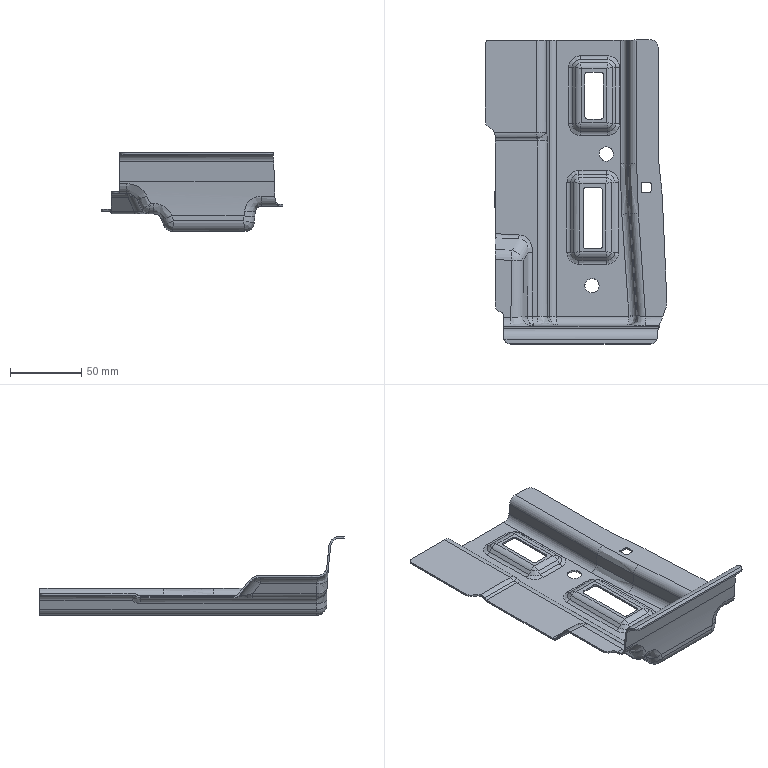Part | 1 solid | 283 faces | box 127.65 x 213.5 x 55.442 mm | volume 39550 mm3 | spline 129 | cylinder 103 | plane 49 | sphere 2 | commonest cylinder face diameters 10 x30 7.6 x11 12.4 x9 4 x8 12.6 x6 15 x6